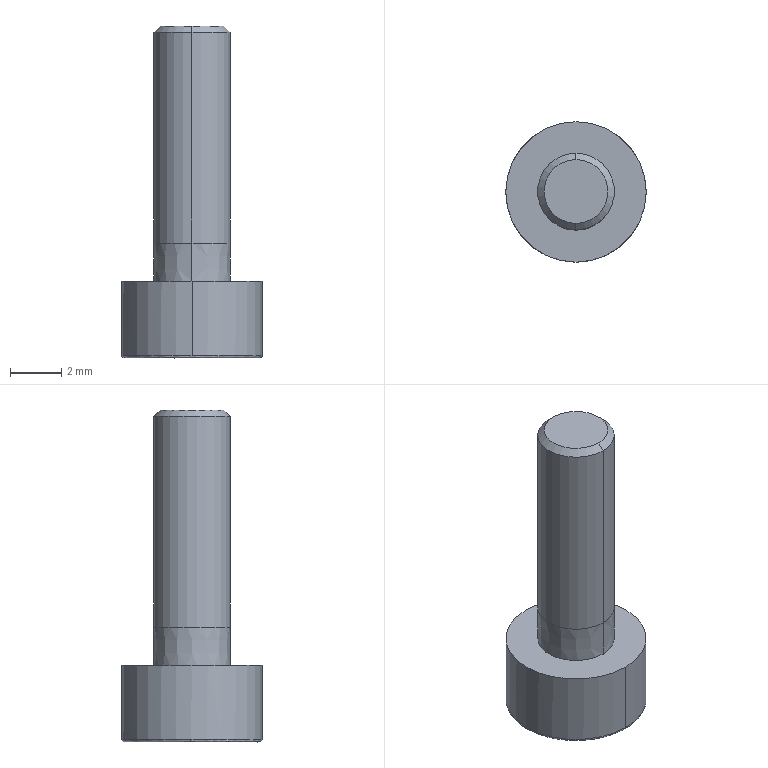Part | SolidWorks | features BaseBody 1 | 1 solid | 20 faces | box 5.5 x 5.5 x 13 mm | volume 134.6 mm3 | plane 10 | cylinder 4 | cone 4 | spline 2 | commonest cylinder face diameters 3 x2 5.5 x2
STEP:
#1=CARTESIAN_POINT('',(510.512,-10.442,230.819));
#2=VERTEX_POINT('',#1);
#3=CARTESIAN_POINT('',(513.262,-13.233,230.819));
#4=VERTEX_POINT('',#3);
#5=CARTESIAN_POINT('',(513.262,-10.483,230.819));
#6=DIRECTION('',(-0.000000003,-0.000000008,1.));
#7=DIRECTION('',(0.,-1.,-0.000000008));
#8=AXIS2_PLACEMENT_3D('',#5,#6,#7);
#9=CIRCLE('',#8,2.75);
#10=EDGE_CURVE('',#2,#4,#9,.T.);
#11=ORIENTED_EDGE('',*,*,#10,.F.);
#12=CARTESIAN_POINT('',(510.612,-10.443,230.719));
#13=VERTEX_POINT('',#12);
#14=CARTESIAN_POINT('',(510.612,-10.443,230.819));
#15=DIRECTION('',(-0.01505,-0.9999,-0.000000008));
#16=DIRECTION('',(-0.9999,0.01505,-0.000000003));
#17=AXIS2_PLACEMENT_3D('',#14,#15,#16);
#18=CIRCLE('',#17,0.1);
#19=EDGE_CURVE('',#2,#13,#18,.T.);
#20=ORIENTED_EDGE('',*,*,#19,.T.);
#21=CARTESIAN_POINT('',(515.911,-10.523,230.719));
#22=VERTEX_POINT('',#21);
#23=CARTESIAN_POINT('',(510.612,-10.443,230.719));
#24=CARTESIAN_POINT('',(510.532,-15.743,230.719));
#25=CARTESIAN_POINT('',(515.831,-15.823,230.719));
#26=CARTESIAN_POINT('',(515.911,-10.523,230.719));
#27=(BOUNDED_CURVE()B_SPLINE_CURVE(3,(#23,#24,#25,#26),.UNSPECIFIED.,.F.,.F.)B_SPLINE_CURVE_WITH_KNOTS((4,4),(0.,1.),.UNSPECIFIED.)CURVE()GEOMETRIC_REPRESENTATION_ITEM()RATIONAL_B_SPLINE_CURVE((1.,0.3333,0.3333,1.))REPRESENTATION_ITEM(''));
#28=EDGE_CURVE('',#13,#22,#27,.T.);
#29=ORIENTED_EDGE('',*,*,#28,.T.);
#30=CARTESIAN_POINT('',(516.011,-10.525,230.819));
#31=VERTEX_POINT('',#30);
#32=CARTESIAN_POINT('',(515.911,-10.523,230.819));
#33=DIRECTION('',(0.01505,0.9999,0.000000008));
#34=DIRECTION('',(0.9999,-0.01505,0.000000003));
#35=AXIS2_PLACEMENT_3D('',#32,#33,#34);
#36=CIRCLE('',#35,0.1);
#37=EDGE_CURVE('',#31,#22,#36,.T.);
#38=ORIENTED_EDGE('',*,*,#37,.F.);
#39=CARTESIAN_POINT('',(513.262,-10.483,230.819));
#40=DIRECTION('',(-0.000000003,-0.000000008,1.));
#41=DIRECTION('',(0.,-1.,-0.000000008));
#42=AXIS2_PLACEMENT_3D('',#39,#40,#41);
#43=CIRCLE('',#42,2.75);
#44=EDGE_CURVE('',#4,#31,#43,.T.);
#45=ORIENTED_EDGE('',*,*,#44,.F.);
#46=EDGE_LOOP('',(#11,#20,#29,#38,#45));
#47=FACE_OUTER_BOUND('',#46,.T.);
#48=CARTESIAN_POINT('',(510.512,-10.442,230.819));
#49=CARTESIAN_POINT('',(510.429,-15.941,230.819));
#50=CARTESIAN_POINT('',(515.928,-16.024,230.819));
#51=CARTESIAN_POINT('',(516.011,-10.525,230.819));
#52=CARTESIAN_POINT('',(510.512,-10.442,230.761));
#53=CARTESIAN_POINT('',(510.429,-15.941,230.761));
#54=CARTESIAN_POINT('',(515.928,-16.024,230.761));
#55=CARTESIAN_POINT('',(516.011,-10.525,230.761));
#56=CARTESIAN_POINT('',(510.553,-10.443,230.719));
#57=CARTESIAN_POINT('',(510.472,-15.859,230.719));
#58=CARTESIAN_POINT('',(515.888,-15.941,230.719));
#59=CARTESIAN_POINT('',(515.97,-10.524,230.719));
#60=CARTESIAN_POINT('',(510.612,-10.443,230.719));
#61=CARTESIAN_POINT('',(510.532,-15.743,230.719));
#62=CARTESIAN_POINT('',(515.831,-15.823,230.719));
#63=CARTESIAN_POINT('',(515.911,-10.523,230.719));
#64=(BOUNDED_SURFACE()B_SPLINE_SURFACE(3,3,((#48,#49,#50,#51),(#52,#53,#54,#55),(#56,#57,#58,#59),(#60,#61,#62,#63)),.UNSPECIFIED.,.F.,.F.,.F.)B_SPLINE_SURFACE_WITH_KNOTS((4,4),(4,4),(0.,1.),(0.,1.),.UNSPECIFIED.)GEOMETRIC_REPRESENTATION_ITEM()RATIONAL_B_SPLINE_SURFACE(((1.,0.3333,0.3333,1.),(0.8047,0.2682,0.2682,0.8047),(0.8047,0.2682,0.2682,0.8047),(1.,0.3333,0.3333,1.)))REPRESENTATION_ITEM('')SURFACE());
#65=ADVANCED_FACE('',(#47),#64,.T.);
#66=CARTESIAN_POINT('',(513.262,-11.983,235.219));
#67=VERTEX_POINT('',#66);
#68=CARTESIAN_POINT('',(513.262,-8.983,235.219));
#69=VERTEX_POINT('',#68);
#70=CARTESIAN_POINT('',(513.262,-10.483,235.219));
#71=DIRECTION('',(-0.000000003,-0.000000008,1.));
#72=DIRECTION('',(0.,-1.,-0.000000008));
#73=AXIS2_PLACEMENT_3D('',#70,#71,#72);
#74=CIRCLE('',#73,1.5);
#75=EDGE_CURVE('',#67,#69,#74,.T.);
#76=ORIENTED_EDGE('',*,*,#75,.T.);
#77=CARTESIAN_POINT('',(513.262,-8.983,243.469));
#78=VERTEX_POINT('',#77);
#79=CARTESIAN_POINT('',(513.262,-8.983,239.344));
#80=DIRECTION('',(-0.000000003,-0.000000008,1.));
#81=VECTOR('',#80,1000.);
#82=LINE('',#79,#81);
#83=EDGE_CURVE('',#69,#78,#82,.T.);
#84=ORIENTED_EDGE('',*,*,#83,.T.);
#85=CARTESIAN_POINT('',(513.262,-11.983,243.469));
#86=VERTEX_POINT('',#85);
#87=CARTESIAN_POINT('',(513.262,-10.483,243.469));
#88=DIRECTION('',(0.000000003,0.000000008,-1.));
#89=DIRECTION('',(0.,-1.,-0.000000008));
#90=AXIS2_PLACEMENT_3D('',#87,#88,#89);
#91=CIRCLE('',#90,1.5);
#92=EDGE_CURVE('',#78,#86,#91,.T.);
#93=ORIENTED_EDGE('',*,*,#92,.T.);
#94=CARTESIAN_POINT('',(513.262,-11.983,239.344));
#95=DIRECTION('',(-0.000000003,-0.000000008,1.));
#96=VECTOR('',#95,1000.);
#97=LINE('',#94,#96);
#98=EDGE_CURVE('',#67,#86,#97,.T.);
#99=ORIENTED_EDGE('',*,*,#98,.F.);
#100=EDGE_LOOP('',(#76,#84,#93,#99));
#101=FACE_OUTER_BOUND('',#100,.T.);
#102=CARTESIAN_POINT('',(513.262,-10.483,239.344));
#103=DIRECTION('',(-0.000000003,-0.000000008,1.));
#104=DIRECTION('',(0.,-1.,-0.000000008));
#105=AXIS2_PLACEMENT_3D('',#102,#103,#104);
#106=CYLINDRICAL_SURFACE('',#105,1.5);
#107=ADVANCED_FACE('',(#101),#106,.T.);
#108=CARTESIAN_POINT('',(513.262,-11.983,233.719));
#109=VERTEX_POINT('',#108);
#110=CARTESIAN_POINT('',(513.262,-8.984,233.719));
#111=VERTEX_POINT('',#110);
#112=CARTESIAN_POINT('',(513.262,-10.483,233.719));
#113=DIRECTION('',(-0.000000003,-0.000000008,1.));
#114=DIRECTION('',(0.,-1.,-0.000000008));
#115=AXIS2_PLACEMENT_3D('',#112,#113,#114);
#116=CIRCLE('',#115,1.499);
#117=EDGE_CURVE('',#109,#111,#116,.T.);
#118=ORIENTED_EDGE('',*,*,#117,.T.);
#119=CARTESIAN_POINT('',(513.262,-8.983,235.219));
#120=DIRECTION('',(-0.000000003,0.0005,1.));
#121=VECTOR('',#120,1000.);
#122=LINE('',#119,#121);
#123=EDGE_CURVE('',#111,#69,#122,.T.);
#124=ORIENTED_EDGE('',*,*,#123,.T.);
#125=ORIENTED_EDGE('',*,*,#75,.F.);
#126=CARTESIAN_POINT('',(513.262,-11.983,235.219));
#127=DIRECTION('',(-0.000000003,-0.0005,1.));
#128=VECTOR('',#127,1000.);
#129=LINE('',#126,#128);
#130=EDGE_CURVE('',#109,#67,#129,.T.);
#131=ORIENTED_EDGE('',*,*,#130,.F.);
#132=EDGE_LOOP('',(#118,#124,#125,#131));
#133=FACE_OUTER_BOUND('',#132,.T.);
#134=CARTESIAN_POINT('',(513.262,-10.483,235.219));
#135=DIRECTION('',(-0.000000003,-0.000000008,1.));
#136=DIRECTION('',(0.,-1.,-0.000000008));
#137=AXIS2_PLACEMENT_3D('',#134,#135,#136);
#138=CONICAL_SURFACE('',#137,1.5,0.0005);
#139=ADVANCED_FACE('',(#133),#138,.T.);
#140=CARTESIAN_POINT('',(513.262,-9.233,243.719));
#141=VERTEX_POINT('',#140);
#142=CARTESIAN_POINT('',(513.262,-11.733,243.719));
#143=VERTEX_POINT('',#142);
#144=CARTESIAN_POINT('',(513.262,-10.483,243.719));
#145=DIRECTION('',(0.000000003,0.000000008,-1.));
#146=DIRECTION('',(0.,1.,0.000000008));
#147=AXIS2_PLACEMENT_3D('',#144,#145,#146);
#148=CIRCLE('',#147,1.25);
#149=EDGE_CURVE('',#141,#143,#148,.T.);
#150=ORIENTED_EDGE('',*,*,#149,.T.);
#151=CARTESIAN_POINT('',(513.262,-11.983,243.469));
#152=DIRECTION('',(0.000000002,-0.7071,-0.7071));
#153=VECTOR('',#152,1000.);
#154=LINE('',#151,#153);
#155=EDGE_CURVE('',#143,#86,#154,.T.);
#156=ORIENTED_EDGE('',*,*,#155,.T.);
#157=ORIENTED_EDGE('',*,*,#92,.F.);
#158=CARTESIAN_POINT('',(513.262,-8.983,243.469));
#159=DIRECTION('',(0.000000002,0.7071,-0.7071));
#160=VECTOR('',#159,1000.);
#161=LINE('',#158,#160);
#162=EDGE_CURVE('',#141,#78,#161,.T.);
#163=ORIENTED_EDGE('',*,*,#162,.F.);
#164=EDGE_LOOP('',(#150,#156,#157,#163));
#165=FACE_OUTER_BOUND('',#164,.T.);
#166=CARTESIAN_POINT('',(513.262,-10.483,243.469));
#167=DIRECTION('',(0.000000003,0.000000008,-1.));
#168=DIRECTION('',(0.,1.,0.000000008));
#169=AXIS2_PLACEMENT_3D('',#166,#167,#168);
#170=CONICAL_SURFACE('',#169,1.5,0.7854);
#171=ADVANCED_FACE('',(#165),#170,.T.);
#172=ORIENTED_EDGE('',*,*,#44,.T.);
#173=CARTESIAN_POINT('',(513.262,-7.733,230.819));
#174=VERTEX_POINT('',#173);
#175=CARTESIAN_POINT('',(513.262,-10.483,230.819));
#176=DIRECTION('',(-0.000000003,-0.000000008,1.));
#177=DIRECTION('',(0.,-1.,-0.000000008));
#178=AXIS2_PLACEMENT_3D('',#175,#176,#177);
#179=CIRCLE('',#178,2.75);
#180=EDGE_CURVE('',#31,#174,#179,.T.);
#181=ORIENTED_EDGE('',*,*,#180,.T.);
#182=CARTESIAN_POINT('',(513.262,-7.733,233.719));
#183=VERTEX_POINT('',#182);
#184=CARTESIAN_POINT('',(513.262,-7.733,232.269));
#185=DIRECTION('',(-0.000000003,-0.000000008,1.));
#186=VECTOR('',#185,1000.);
#187=LINE('',#184,#186);
#188=EDGE_CURVE('',#174,#183,#187,.T.);
#189=ORIENTED_EDGE('',*,*,#188,.T.);
#190=CARTESIAN_POINT('',(513.262,-13.233,233.719));
#191=VERTEX_POINT('',#190);
#192=CARTESIAN_POINT('',(513.262,-10.483,233.719));
#193=DIRECTION('',(-0.000000003,-0.000000008,1.));
#194=DIRECTION('',(0.,-1.,-0.000000008));
#195=AXIS2_PLACEMENT_3D('',#192,#193,#194);
#196=CIRCLE('',#195,2.75);
#197=EDGE_CURVE('',#191,#183,#196,.T.);
#198=ORIENTED_EDGE('',*,*,#197,.F.);
#199=CARTESIAN_POINT('',(513.262,-13.233,232.269));
#200=DIRECTION('',(-0.000000003,-0.000000008,1.));
#201=VECTOR('',#200,1000.);
#202=LINE('',#199,#201);
#203=EDGE_CURVE('',#4,#191,#202,.T.);
#204=ORIENTED_EDGE('',*,*,#203,.F.);
#205=EDGE_LOOP('',(#172,#181,#189,#198,#204));
#206=FACE_OUTER_BOUND('',#205,.T.);
#207=CARTESIAN_POINT('',(513.262,-10.483,232.269));
#208=DIRECTION('',(-0.000000003,-0.000000008,1.));
#209=DIRECTION('',(0.,-1.,-0.000000008));
#210=AXIS2_PLACEMENT_3D('',#207,#208,#209);
#211=CYLINDRICAL_SURFACE('',#210,2.75);
#212=ADVANCED_FACE('',(#206),#211,.T.);
#213=ORIENTED_EDGE('',*,*,#83,.F.);
#214=CARTESIAN_POINT('',(513.262,-10.483,235.219));
#215=DIRECTION('',(-0.000000003,-0.000000008,1.));
#216=DIRECTION('',(0.,-1.,-0.000000008));
#217=AXIS2_PLACEMENT_3D('',#214,#215,#216);
#218=CIRCLE('',#217,1.5);
#219=EDGE_CURVE('',#69,#67,#218,.T.);
#220=ORIENTED_EDGE('',*,*,#219,.T.);
#221=ORIENTED_EDGE('',*,*,#98,.T.);
#222=CARTESIAN_POINT('',(513.262,-10.483,243.469));
#223=DIRECTION('',(0.000000003,0.000000008,-1.));
#224=DIRECTION('',(0.,-1.,-0.000000008));
#225=AXIS2_PLACEMENT_3D('',#222,#223,#224);
#226=CIRCLE('',#225,1.5);
#227=EDGE_CURVE('',#86,#78,#226,.T.);
#228=ORIENTED_EDGE('',*,*,#227,.T.);
#229=EDGE_LOOP('',(#213,#220,#221,#228));
#230=FACE_OUTER_BOUND('',#229,.T.);
#231=CARTESIAN_POINT('',(513.262,-10.483,239.344));
#232=DIRECTION('',(-0.000000003,-0.000000008,1.));
#233=DIRECTION('',(0.,-1.,-0.000000008));
#234=AXIS2_PLACEMENT_3D('',#231,#232,#233);
#235=CYLINDRICAL_SURFACE('',#234,1.5);
#236=ADVANCED_FACE('',(#230),#235,.T.);
#237=ORIENTED_EDGE('',*,*,#123,.F.);
#238=CARTESIAN_POINT('',(513.262,-10.483,233.719));
#239=DIRECTION('',(-0.000000003,-0.000000008,1.));
#240=DIRECTION('',(0.,-1.,-0.000000008));
#241=AXIS2_PLACEMENT_3D('',#238,#239,#240);
#242=CIRCLE('',#241,1.499);
#243=EDGE_CURVE('',#111,#109,#242,.T.);
#244=ORIENTED_EDGE('',*,*,#243,.T.);
#245=ORIENTED_EDGE('',*,*,#130,.T.);
#246=ORIENTED_EDGE('',*,*,#219,.F.);
#247=EDGE_LOOP('',(#237,#244,#245,#246));
#248=FACE_OUTER_BOUND('',#247,.T.);
#249=CARTESIAN_POINT('',(513.262,-10.483,235.219));
#250=DIRECTION('',(-0.000000003,-0.000000008,1.));
#251=DIRECTION('',(0.,-1.,-0.000000008));
#252=AXIS2_PLACEMENT_3D('',#249,#250,#251);
#253=CONICAL_SURFACE('',#252,1.5,0.0005);
#254=ADVANCED_FACE('',(#248),#253,.T.);
#255=ORIENTED_EDGE('',*,*,#155,.F.);
#256=CARTESIAN_POINT('',(513.262,-10.483,243.719));
#257=DIRECTION('',(0.000000003,0.000000008,-1.));
#258=DIRECTION('',(0.,1.,0.000000008));
#259=AXIS2_PLACEMENT_3D('',#256,#257,#258);
#260=CIRCLE('',#259,1.25);
#261=EDGE_CURVE('',#143,#141,#260,.T.);
#262=ORIENTED_EDGE('',*,*,#261,.T.);
#263=ORIENTED_EDGE('',*,*,#162,.T.);
#264=ORIENTED_EDGE('',*,*,#227,.F.);
#265=EDGE_LOOP('',(#255,#262,#263,#264));
#266=FACE_OUTER_BOUND('',#265,.T.);
#267=CARTESIAN_POINT('',(513.262,-10.483,243.469));
#268=DIRECTION('',(0.000000003,0.000000008,-1.));
#269=DIRECTION('',(0.,1.,0.000000008));
#270=AXIS2_PLACEMENT_3D('',#267,#268,#269);
#271=CONICAL_SURFACE('',#270,1.5,0.7854);
#272=ADVANCED_FACE('',(#266),#271,.T.);
#273=ORIENTED_EDGE('',*,*,#117,.F.);
#274=ORIENTED_EDGE('',*,*,#243,.F.);
#275=EDGE_LOOP('',(#273,#274));
#276=FACE_BOUND('',#275,.T.);
#277=ORIENTED_EDGE('',*,*,#197,.T.);
#278=CARTESIAN_POINT('',(513.262,-10.483,233.719));
#279=DIRECTION('',(-0.000000003,-0.000000008,1.));
#280=DIRECTION('',(0.,-1.,-0.000000008));
#281=AXIS2_PLACEMENT_3D('',#278,#279,#280);
#282=CIRCLE('',#281,2.75);
#283=EDGE_CURVE('',#183,#191,#282,.T.);
#284=ORIENTED_EDGE('',*,*,#283,.T.);
#285=EDGE_LOOP('',(#277,#284));
#286=FACE_OUTER_BOUND('',#285,.T.);
#287=CARTESIAN_POINT('',(514.636,-10.504,233.719));
#288=DIRECTION('',(-0.000000003,-0.000000008,1.));
#289=DIRECTION('',(0.,-1.,-0.000000008));
#290=AXIS2_PLACEMENT_3D('',#287,#288,#289);
#291=PLANE('',#290);
#292=ADVANCED_FACE('',(#276,#286),#291,.T.);
#293=ORIENTED_EDGE('',*,*,#149,.F.);
#294=ORIENTED_EDGE('',*,*,#261,.F.);
#295=EDGE_LOOP('',(#293,#294));
#296=FACE_OUTER_BOUND('',#295,.T.);
#297=CARTESIAN_POINT('',(513.886,-10.493,243.719));
#298=DIRECTION('',(-0.000000003,-0.000000008,1.));
#299=DIRECTION('',(0.,-1.,-0.000000008));
#300=AXIS2_PLACEMENT_3D('',#297,#298,#299);
#301=PLANE('',#300);
#302=ADVANCED_FACE('',(#296),#301,.T.);
#303=ORIENTED_EDGE('',*,*,#188,.F.);
#304=CARTESIAN_POINT('',(513.262,-10.483,230.819));
#305=DIRECTION('',(-0.000000003,-0.000000008,1.));
#306=DIRECTION('',(0.,-1.,-0.000000008));
#307=AXIS2_PLACEMENT_3D('',#304,#305,#306);
#308=CIRCLE('',#307,2.75);
#309=EDGE_CURVE('',#174,#2,#308,.T.);
#310=ORIENTED_EDGE('',*,*,#309,.T.);
#311=ORIENTED_EDGE('',*,*,#10,.T.);
#312=ORIENTED_EDGE('',*,*,#203,.T.);
#313=ORIENTED_EDGE('',*,*,#283,.F.);
#314=EDGE_LOOP('',(#303,#310,#311,#312,#313));
#315=FACE_OUTER_BOUND('',#314,.T.);
#316=CARTESIAN_POINT('',(513.262,-10.483,232.269));
#317=DIRECTION('',(-0.000000003,-0.000000008,1.));
#318=DIRECTION('',(0.,-1.,-0.000000008));
#319=AXIS2_PLACEMENT_3D('',#316,#317,#318);
#320=CYLINDRICAL_SURFACE('',#319,2.75);
#321=ADVANCED_FACE('',(#315),#320,.T.);
#322=ORIENTED_EDGE('',*,*,#19,.F.);
#323=ORIENTED_EDGE('',*,*,#309,.F.);
#324=ORIENTED_EDGE('',*,*,#180,.F.);
#325=ORIENTED_EDGE('',*,*,#37,.T.);
#326=CARTESIAN_POINT('',(515.911,-10.523,230.719));
#327=CARTESIAN_POINT('',(515.991,-5.224,230.719));
#328=CARTESIAN_POINT('',(510.692,-5.144,230.719));
#329=CARTESIAN_POINT('',(510.612,-10.443,230.719));
#330=(BOUNDED_CURVE()B_SPLINE_CURVE(3,(#326,#327,#328,#329),.UNSPECIFIED.,.F.,.F.)B_SPLINE_CURVE_WITH_KNOTS((4,4),(0.,1.),.UNSPECIFIED.)CURVE()GEOMETRIC_REPRESENTATION_ITEM()RATIONAL_B_SPLINE_CURVE((1.,0.3333,0.3333,1.))REPRESENTATION_ITEM(''));
#331=EDGE_CURVE('',#22,#13,#330,.T.);
#332=ORIENTED_EDGE('',*,*,#331,.T.);
#333=EDGE_LOOP('',(#322,#323,#324,#325,#332));
#334=FACE_OUTER_BOUND('',#333,.T.);
#335=CARTESIAN_POINT('',(516.011,-10.525,230.819));
#336=CARTESIAN_POINT('',(516.094,-5.025,230.819));
#337=CARTESIAN_POINT('',(510.595,-4.943,230.819));
#338=CARTESIAN_POINT('',(510.512,-10.442,230.819));
#339=CARTESIAN_POINT('',(516.011,-10.525,230.761));
#340=CARTESIAN_POINT('',(516.094,-5.025,230.761));
#341=CARTESIAN_POINT('',(510.595,-4.943,230.761));
#342=CARTESIAN_POINT('',(510.512,-10.442,230.761));
#343=CARTESIAN_POINT('',(515.97,-10.524,230.719));
#344=CARTESIAN_POINT('',(516.051,-5.108,230.719));
#345=CARTESIAN_POINT('',(510.635,-5.026,230.719));
#346=CARTESIAN_POINT('',(510.553,-10.443,230.719));
#347=CARTESIAN_POINT('',(515.911,-10.523,230.719));
#348=CARTESIAN_POINT('',(515.991,-5.224,230.719));
#349=CARTESIAN_POINT('',(510.692,-5.144,230.719));
#350=CARTESIAN_POINT('',(510.612,-10.443,230.719));
#351=(BOUNDED_SURFACE()B_SPLINE_SURFACE(3,3,((#335,#336,#337,#338),(#339,#340,#341,#342),(#343,#344,#345,#346),(#347,#348,#349,#350)),.UNSPECIFIED.,.F.,.F.,.F.)B_SPLINE_SURFACE_WITH_KNOTS((4,4),(4,4),(0.,1.),(0.,1.),.UNSPECIFIED.)GEOMETRIC_REPRESENTATION_ITEM()RATIONAL_B_SPLINE_SURFACE(((1.,0.3333,0.3333,1.),(0.8047,0.2682,0.2682,0.8047),(0.8047,0.2682,0.2682,0.8047),(1.,0.3333,0.3333,1.)))REPRESENTATION_ITEM('')SURFACE());
#352=ADVANCED_FACE('',(#334),#351,.T.);
#353=ORIENTED_EDGE('',*,*,#28,.F.);
#354=ORIENTED_EDGE('',*,*,#331,.F.);
#355=EDGE_LOOP('',(#353,#354));
#356=FACE_OUTER_BOUND('',#355,.T.);
#357=CARTESIAN_POINT('',(512.559,-9.223,230.719));
#358=VERTEX_POINT('',#357);
#359=CARTESIAN_POINT('',(511.818,-10.462,230.719));
#360=VERTEX_POINT('',#359);
#361=CARTESIAN_POINT('',(512.559,-9.223,230.719));
#362=DIRECTION('',(-0.513,-0.8584,-0.000000009));
#363=VECTOR('',#362,1000.);
#364=LINE('',#361,#363);
#365=EDGE_CURVE('',#358,#360,#364,.T.);
#366=ORIENTED_EDGE('',*,*,#365,.T.);
#367=CARTESIAN_POINT('',(512.521,-11.722,230.719));
#368=VERTEX_POINT('',#367);
#369=CARTESIAN_POINT('',(511.818,-10.462,230.719));
#370=DIRECTION('',(0.4869,-0.8735,-0.000000006));
#371=VECTOR('',#370,1000.);
#372=LINE('',#369,#371);
#373=EDGE_CURVE('',#360,#368,#372,.T.);
#374=ORIENTED_EDGE('',*,*,#373,.T.);
#375=CARTESIAN_POINT('',(513.964,-11.744,230.719));
#376=VERTEX_POINT('',#375);
#377=CARTESIAN_POINT('',(512.521,-11.722,230.719));
#378=DIRECTION('',(0.9999,-0.01505,0.000000003));
#379=VECTOR('',#378,1000.);
#380=LINE('',#377,#379);
#381=EDGE_CURVE('',#368,#376,#380,.T.);
#382=ORIENTED_EDGE('',*,*,#381,.T.);
#383=CARTESIAN_POINT('',(514.705,-10.505,230.719));
#384=VERTEX_POINT('',#383);
#385=CARTESIAN_POINT('',(513.964,-11.744,230.719));
#386=DIRECTION('',(0.513,0.8584,0.000000009));
#387=VECTOR('',#386,1000.);
#388=LINE('',#385,#387);
#389=EDGE_CURVE('',#376,#384,#388,.T.);
#390=ORIENTED_EDGE('',*,*,#389,.T.);
#391=CARTESIAN_POINT('',(514.002,-9.244,230.719));
#392=VERTEX_POINT('',#391);
#393=CARTESIAN_POINT('',(514.705,-10.505,230.719));
#394=DIRECTION('',(-0.4869,0.8735,0.000000006));
#395=VECTOR('',#394,1000.);
#396=LINE('',#393,#395);
#397=EDGE_CURVE('',#384,#392,#396,.T.);
#398=ORIENTED_EDGE('',*,*,#397,.T.);
#399=CARTESIAN_POINT('',(514.002,-9.244,230.719));
#400=DIRECTION('',(-0.9999,0.01505,-0.000000003));
#401=VECTOR('',#400,1000.);
#402=LINE('',#399,#401);
#403=EDGE_CURVE('',#392,#358,#402,.T.);
#404=ORIENTED_EDGE('',*,*,#403,.T.);
#405=EDGE_LOOP('',(#366,#374,#382,#390,#398,#404));
#406=FACE_BOUND('',#405,.T.);
#407=CARTESIAN_POINT('',(514.586,-10.503,230.719));
#408=DIRECTION('',(0.000000003,0.000000008,-1.));
#409=DIRECTION('',(0.,1.,0.000000008));
#410=AXIS2_PLACEMENT_3D('',#407,#408,#409);
#411=PLANE('',#410);
#412=ADVANCED_FACE('',(#356,#406),#411,.T.);
#413=CARTESIAN_POINT('',(512.521,-11.722,232.019));
#414=VERTEX_POINT('',#413);
#415=CARTESIAN_POINT('',(512.521,-11.722,230.719));
#416=DIRECTION('',(-0.000000006,-0.000000003,1.));
#417=VECTOR('',#416,1000.);
#418=LINE('',#415,#417);
#419=EDGE_CURVE('',#368,#414,#418,.T.);
#420=ORIENTED_EDGE('',*,*,#419,.F.);
#421=ORIENTED_EDGE('',*,*,#373,.F.);
#422=CARTESIAN_POINT('',(511.818,-10.462,232.019));
#423=VERTEX_POINT('',#422);
#424=CARTESIAN_POINT('',(511.818,-10.462,230.719));
#425=DIRECTION('',(0.000000006,0.000000003,-1.));
#426=VECTOR('',#425,1000.);
#427=LINE('',#424,#426);
#428=EDGE_CURVE('',#423,#360,#427,.T.);
#429=ORIENTED_EDGE('',*,*,#428,.F.);
#430=CARTESIAN_POINT('',(512.521,-11.722,232.019));
#431=DIRECTION('',(-0.4869,0.8735,0.));
#432=VECTOR('',#431,1000.);
#433=LINE('',#430,#432);
#434=EDGE_CURVE('',#414,#423,#433,.T.);
#435=ORIENTED_EDGE('',*,*,#434,.F.);
#436=EDGE_LOOP('',(#420,#421,#429,#435));
#437=FACE_OUTER_BOUND('',#436,.T.);
#438=CARTESIAN_POINT('',(512.521,-11.722,230.719));
#439=DIRECTION('',(-0.8735,-0.4869,-0.000000007));
#440=DIRECTION('',(0.4869,-0.8735,0.));
#441=AXIS2_PLACEMENT_3D('',#438,#439,#440);
#442=PLANE('',#441);
#443=ADVANCED_FACE('',(#437),#442,.F.);
#444=ORIENTED_EDGE('',*,*,#428,.T.);
#445=ORIENTED_EDGE('',*,*,#365,.F.);
#446=CARTESIAN_POINT('',(512.559,-9.223,232.019));
#447=VERTEX_POINT('',#446);
#448=CARTESIAN_POINT('',(512.559,-9.223,230.719));
#449=DIRECTION('',(-0.000000002,0.000000001,-1.));
#450=VECTOR('',#449,1000.);
#451=LINE('',#448,#450);
#452=EDGE_CURVE('',#447,#358,#451,.T.);
#453=ORIENTED_EDGE('',*,*,#452,.F.);
#454=CARTESIAN_POINT('',(511.818,-10.462,232.019));
#455=DIRECTION('',(0.513,0.8584,0.));
#456=VECTOR('',#455,1000.);
#457=LINE('',#454,#456);
#458=EDGE_CURVE('',#423,#447,#457,.T.);
#459=ORIENTED_EDGE('',*,*,#458,.F.);
#460=EDGE_LOOP('',(#444,#445,#453,#459));
#461=FACE_OUTER_BOUND('',#460,.T.);
#462=CARTESIAN_POINT('',(511.818,-10.462,230.719));
#463=DIRECTION('',(-0.8584,0.513,0.000000002));
#464=DIRECTION('',(-0.513,-0.8584,0.));
#465=AXIS2_PLACEMENT_3D('',#462,#463,#464);
#466=PLANE('',#465);
#467=ADVANCED_FACE('',(#461),#466,.F.);
#468=ORIENTED_EDGE('',*,*,#452,.T.);
#469=ORIENTED_EDGE('',*,*,#403,.F.);
#470=CARTESIAN_POINT('',(514.002,-9.244,232.019));
#471=VERTEX_POINT('',#470);
#472=CARTESIAN_POINT('',(514.002,-9.244,230.719));
#473=DIRECTION('',(0.,0.000000008,-1.));
#474=VECTOR('',#473,1000.);
#475=LINE('',#472,#474);
#476=EDGE_CURVE('',#471,#392,#475,.T.);
#477=ORIENTED_EDGE('',*,*,#476,.F.);
#478=CARTESIAN_POINT('',(512.559,-9.223,232.019));
#479=DIRECTION('',(0.9999,-0.01505,0.));
#480=VECTOR('',#479,1000.);
#481=LINE('',#478,#480);
#482=EDGE_CURVE('',#447,#471,#481,.T.);
#483=ORIENTED_EDGE('',*,*,#482,.F.);
#484=EDGE_LOOP('',(#468,#469,#477,#483));
#485=FACE_OUTER_BOUND('',#484,.T.);
#486=CARTESIAN_POINT('',(512.559,-9.223,230.719));
#487=DIRECTION('',(0.01505,0.9999,0.000000008));
#488=DIRECTION('',(-0.9999,0.01505,0.));
#489=AXIS2_PLACEMENT_3D('',#486,#487,#488);
#490=PLANE('',#489);
#491=ADVANCED_FACE('',(#485),#490,.F.);
#492=ORIENTED_EDGE('',*,*,#476,.T.);
#493=ORIENTED_EDGE('',*,*,#397,.F.);
#494=CARTESIAN_POINT('',(514.705,-10.505,232.019));
#495=VERTEX_POINT('',#494);
#496=CARTESIAN_POINT('',(514.705,-10.505,230.719));
#497=DIRECTION('',(0.000000006,0.000000003,-1.));
#498=VECTOR('',#497,1000.);
#499=LINE('',#496,#498);
#500=EDGE_CURVE('',#495,#384,#499,.T.);
#501=ORIENTED_EDGE('',*,*,#500,.F.);
#502=CARTESIAN_POINT('',(514.002,-9.244,232.019));
#503=DIRECTION('',(0.4869,-0.8735,0.));
#504=VECTOR('',#503,1000.);
#505=LINE('',#502,#504);
#506=EDGE_CURVE('',#471,#495,#505,.T.);
#507=ORIENTED_EDGE('',*,*,#506,.F.);
#508=EDGE_LOOP('',(#492,#493,#501,#507));
#509=FACE_OUTER_BOUND('',#508,.T.);
#510=CARTESIAN_POINT('',(514.002,-9.244,230.719));
#511=DIRECTION('',(0.8735,0.4869,0.000000007));
#512=DIRECTION('',(-0.4869,0.8735,0.));
#513=AXIS2_PLACEMENT_3D('',#510,#511,#512);
#514=PLANE('',#513);
#515=ADVANCED_FACE('',(#509),#514,.F.);
#516=ORIENTED_EDGE('',*,*,#500,.T.);
#517=ORIENTED_EDGE('',*,*,#389,.F.);
#518=CARTESIAN_POINT('',(513.964,-11.744,232.019));
#519=VERTEX_POINT('',#518);
#520=CARTESIAN_POINT('',(513.964,-11.744,230.719));
#521=DIRECTION('',(-0.000000002,0.000000001,-1.));
#522=VECTOR('',#521,1000.);
#523=LINE('',#520,#522);
#524=EDGE_CURVE('',#519,#376,#523,.T.);
#525=ORIENTED_EDGE('',*,*,#524,.F.);
#526=CARTESIAN_POINT('',(514.705,-10.505,232.019));
#527=DIRECTION('',(-0.513,-0.8584,0.));
#528=VECTOR('',#527,1000.);
#529=LINE('',#526,#528);
#530=EDGE_CURVE('',#495,#519,#529,.T.);
#531=ORIENTED_EDGE('',*,*,#530,.F.);
#532=EDGE_LOOP('',(#516,#517,#525,#531));
#533=FACE_OUTER_BOUND('',#532,.T.);
#534=CARTESIAN_POINT('',(514.705,-10.505,230.719));
#535=DIRECTION('',(0.8584,-0.513,-0.000000002));
#536=DIRECTION('',(0.513,0.8584,0.));
#537=AXIS2_PLACEMENT_3D('',#534,#535,#536);
#538=PLANE('',#537);
#539=ADVANCED_FACE('',(#533),#538,.F.);
#540=ORIENTED_EDGE('',*,*,#524,.T.);
#541=ORIENTED_EDGE('',*,*,#381,.F.);
#542=ORIENTED_EDGE('',*,*,#419,.T.);
#543=CARTESIAN_POINT('',(513.964,-11.744,232.019));
#544=DIRECTION('',(-0.9999,0.01505,0.));
#545=VECTOR('',#544,1000.);
#546=LINE('',#543,#545);
#547=EDGE_CURVE('',#519,#414,#546,.T.);
#548=ORIENTED_EDGE('',*,*,#547,.F.);
#549=EDGE_LOOP('',(#540,#541,#542,#548));
#550=FACE_OUTER_BOUND('',#549,.T.);
#551=CARTESIAN_POINT('',(513.964,-11.744,230.719));
#552=DIRECTION('',(-0.01505,-0.9999,-0.000000008));
#553=DIRECTION('',(0.9999,-0.01505,0.));
#554=AXIS2_PLACEMENT_3D('',#551,#552,#553);
#555=PLANE('',#554);
#556=ADVANCED_FACE('',(#550),#555,.F.);
#557=ORIENTED_EDGE('',*,*,#506,.T.);
#558=ORIENTED_EDGE('',*,*,#530,.T.);
#559=ORIENTED_EDGE('',*,*,#547,.T.);
#560=ORIENTED_EDGE('',*,*,#434,.T.);
#561=ORIENTED_EDGE('',*,*,#458,.T.);
#562=ORIENTED_EDGE('',*,*,#482,.T.);
#563=EDGE_LOOP('',(#557,#558,#559,#560,#561,#562));
#564=FACE_OUTER_BOUND('',#563,.T.);
#565=CARTESIAN_POINT('',(513.262,-10.483,232.019));
#566=DIRECTION('',(0.000000003,0.000000008,-1.));
#567=DIRECTION('',(0.,1.,0.000000008));
#568=AXIS2_PLACEMENT_3D('',#565,#566,#567);
#569=PLANE('',#568);
#570=ADVANCED_FACE('',(#564),#569,.T.);
#571=CLOSED_SHELL('',(#65,#107,#139,#171,#212,#236,#254,#272,#292,#302,#321,#352,#412,#443,#467,#491,#515,#539,#556,#570));
#572=MANIFOLD_SOLID_BREP('',#571);
#573=CARTESIAN_POINT('',(0.,0.,0.));
#574=DIRECTION('',(0.,0.,1.));
#575=DIRECTION('',(1.,0.,0.));
#576=AXIS2_PLACEMENT_3D('',#573,#574,#575);
#577=(LENGTH_UNIT()NAMED_UNIT(*)SI_UNIT(.MILLI.,.METRE.));
#578=UNCERTAINTY_MEASURE_WITH_UNIT(LENGTH_MEASURE(0.00001),#577,'','');
#579=(NAMED_UNIT(*)PLANE_ANGLE_UNIT()SI_UNIT($,.RADIAN.));
#580=(NAMED_UNIT(*)SI_UNIT($,.STERADIAN.)SOLID_ANGLE_UNIT());
#581=(GEOMETRIC_REPRESENTATION_CONTEXT(3)GLOBAL_UNCERTAINTY_ASSIGNED_CONTEXT((#578))GLOBAL_UNIT_ASSIGNED_CONTEXT((#577,#579,#580))REPRESENTATION_CONTEXT('',''));
#582=ADVANCED_BREP_SHAPE_REPRESENTATION('',(#572,#576),#581);